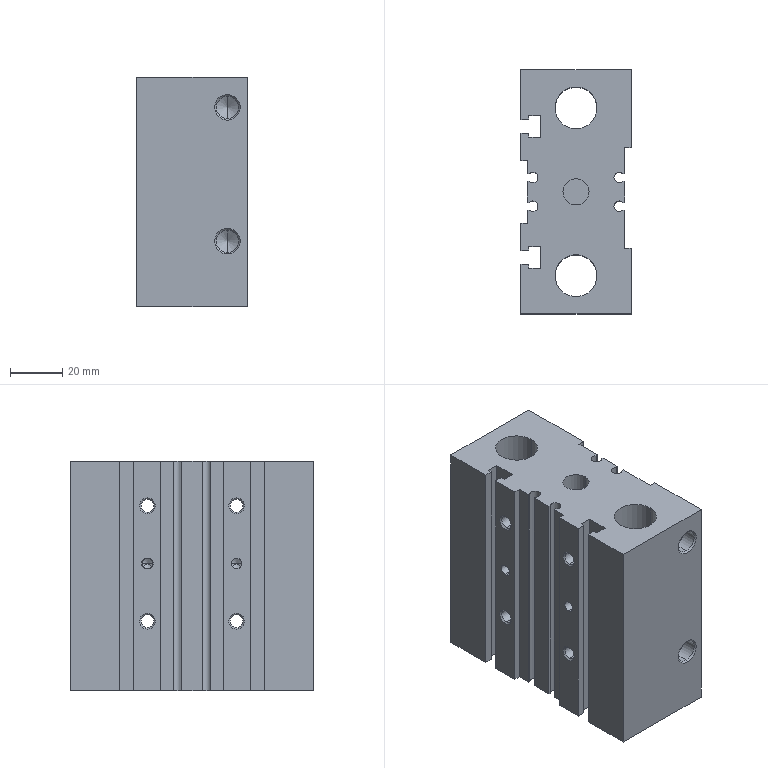Part | SolidWorks | features BaseBody 1 | 1 solid | 178 faces | box 42 x 93 x 87.5 mm | volume 243937 mm3 | cylinder 66 | plane 64 | cone 48 | commonest cylinder face diameters 4.917 x16 4 x12 5.4 x8 8.566 x8 9.5 x8 4.05 x6